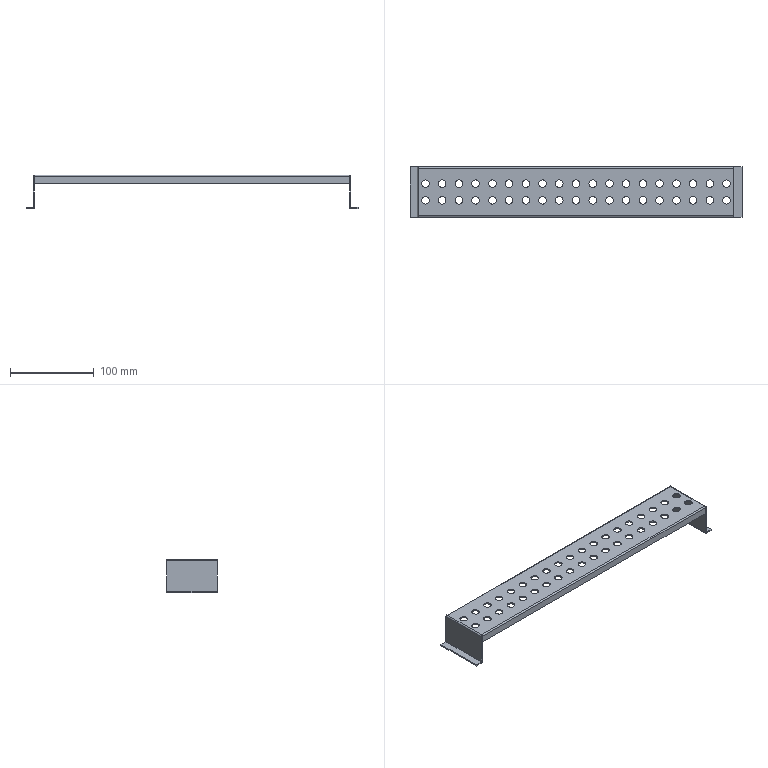Part | SolidWorks | features EdgeFlange 3, FlatPattern 1, ICE 1, SMBaseFlange 1, SheetMetal 1 | 1 solid | 134 faces | box 397 x 60 x 40 mm | volume 48098 mm3 | cylinder 88 | plane 46 | commonest cylinder face diameters 9 x76 0.2 x6 3.2 x6